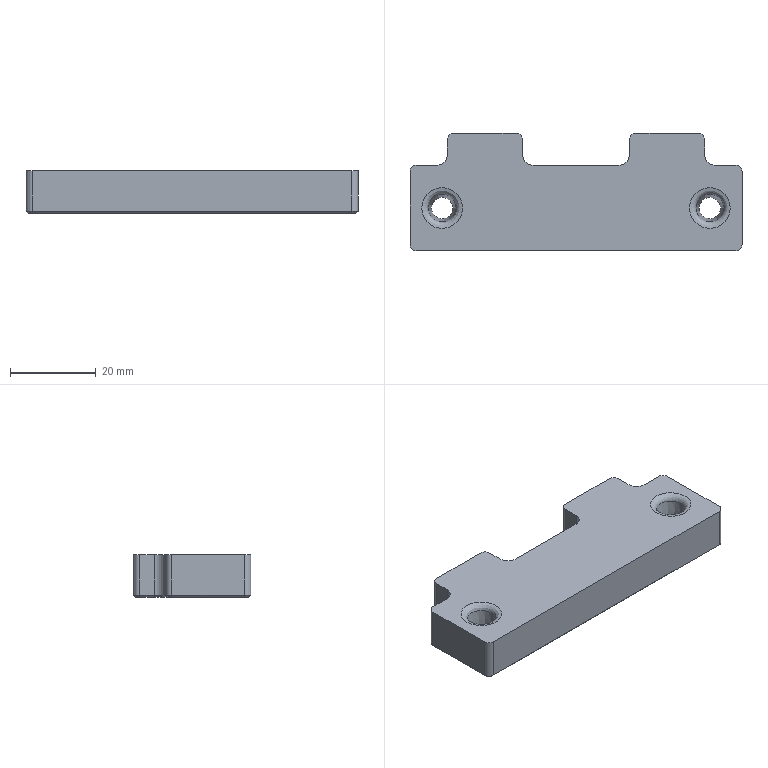Part | NX | features BLEND 3, DATUM_CSYS 3, EXTRUDE 2, SKETCH 2, CHAMFER 1, DRAFT 1, SCALE 1 | 1 solid | 54 faces | box 77.5 x 27.5 x 10 mm | volume 17549 mm3 | plane 26 | cone 14 | cylinder 12 | torus 2 | commonest cylinder face diameters 3 x8 5 x4
STEP:
#1=CARTESIAN_POINT('',(-38.75,8.5,10.));
#2=VERTEX_POINT('',#1);
#3=CARTESIAN_POINT('',(-38.75,8.5,0.5));
#4=VERTEX_POINT('',#3);
#5=CARTESIAN_POINT('',(-38.75,8.5,10.));
#6=DIRECTION('',(0.,0.,-1.));
#7=VECTOR('',#6,1000.);
#8=LINE('',#5,#7);
#9=EDGE_CURVE('',#2,#4,#8,.T.);
#10=ORIENTED_EDGE('',*,*,#9,.T.);
#11=CARTESIAN_POINT('',(-38.75,-8.5,0.5));
#12=VERTEX_POINT('',#11);
#13=CARTESIAN_POINT('',(-38.75,10.,0.5));
#14=DIRECTION('',(0.,-1.,0.));
#15=VECTOR('',#14,1000.);
#16=LINE('',#13,#15);
#17=EDGE_CURVE('',#4,#12,#16,.T.);
#18=ORIENTED_EDGE('',*,*,#17,.T.);
#19=CARTESIAN_POINT('',(-38.75,-8.5,10.));
#20=VERTEX_POINT('',#19);
#21=CARTESIAN_POINT('',(-38.75,-8.5,10.));
#22=DIRECTION('',(0.,0.,-1.));
#23=VECTOR('',#22,1000.);
#24=LINE('',#21,#23);
#25=EDGE_CURVE('',#12,#20,#24,.F.);
#26=ORIENTED_EDGE('',*,*,#25,.T.);
#27=CARTESIAN_POINT('',(-38.75,10.,10.));
#28=DIRECTION('',(0.,-1.,0.));
#29=VECTOR('',#28,1000.);
#30=LINE('',#27,#29);
#31=EDGE_CURVE('',#2,#20,#30,.T.);
#32=ORIENTED_EDGE('',*,*,#31,.F.);
#33=EDGE_LOOP('',(#10,#18,#26,#32));
#34=FACE_BOUND('',#33,.T.);
#35=CARTESIAN_POINT('',(-38.75,10.,10.));
#36=DIRECTION('',(1.,0.,0.));
#37=DIRECTION('',(0.,0.,-1.));
#38=AXIS2_PLACEMENT_3D('',#35,#36,#37);
#39=PLANE('',#38);
#40=ADVANCED_FACE('',(#34),#39,.F.);
#41=CARTESIAN_POINT('',(-37.25,-10.,10.));
#42=VERTEX_POINT('',#41);
#43=CARTESIAN_POINT('',(-37.25,-10.,0.5));
#44=VERTEX_POINT('',#43);
#45=CARTESIAN_POINT('',(-37.25,-10.,10.));
#46=DIRECTION('',(0.,0.,-1.));
#47=VECTOR('',#46,1000.);
#48=LINE('',#45,#47);
#49=EDGE_CURVE('',#42,#44,#48,.T.);
#50=ORIENTED_EDGE('',*,*,#49,.T.);
#51=CARTESIAN_POINT('',(37.25,-10.,0.5));
#52=VERTEX_POINT('',#51);
#53=CARTESIAN_POINT('',(-38.75,-10.,0.5));
#54=DIRECTION('',(1.,0.,0.));
#55=VECTOR('',#54,1000.);
#56=LINE('',#53,#55);
#57=EDGE_CURVE('',#44,#52,#56,.T.);
#58=ORIENTED_EDGE('',*,*,#57,.T.);
#59=CARTESIAN_POINT('',(37.25,-10.,10.));
#60=VERTEX_POINT('',#59);
#61=CARTESIAN_POINT('',(37.25,-10.,10.));
#62=DIRECTION('',(0.,0.,-1.));
#63=VECTOR('',#62,1000.);
#64=LINE('',#61,#63);
#65=EDGE_CURVE('',#52,#60,#64,.F.);
#66=ORIENTED_EDGE('',*,*,#65,.T.);
#67=CARTESIAN_POINT('',(-38.75,-10.,10.));
#68=DIRECTION('',(1.,0.,0.));
#69=VECTOR('',#68,1000.);
#70=LINE('',#67,#69);
#71=EDGE_CURVE('',#42,#60,#70,.T.);
#72=ORIENTED_EDGE('',*,*,#71,.F.);
#73=EDGE_LOOP('',(#50,#58,#66,#72));
#74=FACE_BOUND('',#73,.T.);
#75=CARTESIAN_POINT('',(-38.75,-10.,10.));
#76=DIRECTION('',(0.,1.,0.));
#77=DIRECTION('',(0.,0.,1.));
#78=AXIS2_PLACEMENT_3D('',#75,#76,#77);
#79=PLANE('',#78);
#80=ADVANCED_FACE('',(#74),#79,.F.);
#81=CARTESIAN_POINT('',(38.75,-8.5,10.));
#82=VERTEX_POINT('',#81);
#83=CARTESIAN_POINT('',(38.75,-8.5,0.5));
#84=VERTEX_POINT('',#83);
#85=CARTESIAN_POINT('',(38.75,-8.5,10.));
#86=DIRECTION('',(0.,0.,-1.));
#87=VECTOR('',#86,1000.);
#88=LINE('',#85,#87);
#89=EDGE_CURVE('',#82,#84,#88,.T.);
#90=ORIENTED_EDGE('',*,*,#89,.T.);
#91=CARTESIAN_POINT('',(38.75,8.5,0.5));
#92=VERTEX_POINT('',#91);
#93=CARTESIAN_POINT('',(38.75,-10.,0.5));
#94=DIRECTION('',(0.,1.,0.));
#95=VECTOR('',#94,1000.);
#96=LINE('',#93,#95);
#97=EDGE_CURVE('',#84,#92,#96,.T.);
#98=ORIENTED_EDGE('',*,*,#97,.T.);
#99=CARTESIAN_POINT('',(38.75,8.5,10.));
#100=VERTEX_POINT('',#99);
#101=CARTESIAN_POINT('',(38.75,8.5,10.));
#102=DIRECTION('',(0.,0.,-1.));
#103=VECTOR('',#102,1000.);
#104=LINE('',#101,#103);
#105=EDGE_CURVE('',#92,#100,#104,.F.);
#106=ORIENTED_EDGE('',*,*,#105,.T.);
#107=CARTESIAN_POINT('',(38.75,-10.,10.));
#108=DIRECTION('',(0.,1.,0.));
#109=VECTOR('',#108,1000.);
#110=LINE('',#107,#109);
#111=EDGE_CURVE('',#82,#100,#110,.T.);
#112=ORIENTED_EDGE('',*,*,#111,.F.);
#113=EDGE_LOOP('',(#90,#98,#106,#112));
#114=FACE_BOUND('',#113,.T.);
#115=CARTESIAN_POINT('',(38.75,-10.,10.));
#116=DIRECTION('',(-1.,0.,0.));
#117=DIRECTION('',(0.,0.,1.));
#118=AXIS2_PLACEMENT_3D('',#115,#116,#117);
#119=PLANE('',#118);
#120=ADVANCED_FACE('',(#114),#119,.F.);
#121=CARTESIAN_POINT('',(37.25,10.,10.));
#122=VERTEX_POINT('',#121);
#123=CARTESIAN_POINT('',(37.25,10.,0.5));
#124=VERTEX_POINT('',#123);
#125=CARTESIAN_POINT('',(37.25,10.,10.));
#126=DIRECTION('',(0.,0.,-1.));
#127=VECTOR('',#126,1000.);
#128=LINE('',#125,#127);
#129=EDGE_CURVE('',#122,#124,#128,.T.);
#130=ORIENTED_EDGE('',*,*,#129,.T.);
#131=CARTESIAN_POINT('',(32.5,10.,0.5));
#132=VERTEX_POINT('',#131);
#133=CARTESIAN_POINT('',(38.75,10.,0.5));
#134=DIRECTION('',(-1.,0.,0.));
#135=VECTOR('',#134,1000.);
#136=LINE('',#133,#135);
#137=EDGE_CURVE('',#124,#132,#136,.T.);
#138=ORIENTED_EDGE('',*,*,#137,.T.);
#139=CARTESIAN_POINT('',(32.5,10.,10.));
#140=VERTEX_POINT('',#139);
#141=CARTESIAN_POINT('',(32.5,10.,10.));
#142=DIRECTION('',(0.,0.,-1.));
#143=VECTOR('',#142,1000.);
#144=LINE('',#141,#143);
#145=EDGE_CURVE('',#132,#140,#144,.F.);
#146=ORIENTED_EDGE('',*,*,#145,.T.);
#147=CARTESIAN_POINT('',(38.75,10.,10.));
#148=DIRECTION('',(-1.,0.,0.));
#149=VECTOR('',#148,1000.);
#150=LINE('',#147,#149);
#151=EDGE_CURVE('',#122,#140,#150,.T.);
#152=ORIENTED_EDGE('',*,*,#151,.F.);
#153=EDGE_LOOP('',(#130,#138,#146,#152));
#154=FACE_BOUND('',#153,.T.);
#155=CARTESIAN_POINT('',(38.75,10.,10.));
#156=DIRECTION('',(0.,-1.,0.));
#157=DIRECTION('',(1.,0.,0.));
#158=AXIS2_PLACEMENT_3D('',#155,#156,#157);
#159=PLANE('',#158);
#160=ADVANCED_FACE('',(#154),#159,.F.);
#161=CARTESIAN_POINT('',(30.,12.5,10.));
#162=VERTEX_POINT('',#161);
#163=CARTESIAN_POINT('',(30.,12.5,0.5));
#164=VERTEX_POINT('',#163);
#165=CARTESIAN_POINT('',(30.,12.5,0.));
#166=DIRECTION('',(0.,0.,-1.));
#167=VECTOR('',#166,1000.);
#168=LINE('',#165,#167);
#169=EDGE_CURVE('',#162,#164,#168,.T.);
#170=ORIENTED_EDGE('',*,*,#169,.T.);
#171=CARTESIAN_POINT('',(30.,16.,0.5));
#172=VERTEX_POINT('',#171);
#173=CARTESIAN_POINT('',(30.,10.,0.5));
#174=DIRECTION('',(0.,1.,0.));
#175=VECTOR('',#174,1000.);
#176=LINE('',#173,#175);
#177=EDGE_CURVE('',#164,#172,#176,.T.);
#178=ORIENTED_EDGE('',*,*,#177,.T.);
#179=CARTESIAN_POINT('',(30.,16.,10.));
#180=VERTEX_POINT('',#179);
#181=CARTESIAN_POINT('',(30.,16.,10.));
#182=DIRECTION('',(0.,0.,-1.));
#183=VECTOR('',#182,1000.);
#184=LINE('',#181,#183);
#185=EDGE_CURVE('',#172,#180,#184,.F.);
#186=ORIENTED_EDGE('',*,*,#185,.T.);
#187=CARTESIAN_POINT('',(30.,10.,10.));
#188=DIRECTION('',(0.,1.,0.));
#189=VECTOR('',#188,1000.);
#190=LINE('',#187,#189);
#191=EDGE_CURVE('',#162,#180,#190,.T.);
#192=ORIENTED_EDGE('',*,*,#191,.F.);
#193=EDGE_LOOP('',(#170,#178,#186,#192));
#194=FACE_BOUND('',#193,.T.);
#195=CARTESIAN_POINT('',(30.,10.,10.));
#196=DIRECTION('',(-1.,0.,0.));
#197=DIRECTION('',(0.,0.,1.));
#198=AXIS2_PLACEMENT_3D('',#195,#196,#197);
#199=PLANE('',#198);
#200=ADVANCED_FACE('',(#194),#199,.F.);
#201=CARTESIAN_POINT('',(28.5,17.5,10.));
#202=VERTEX_POINT('',#201);
#203=CARTESIAN_POINT('',(28.5,17.5,0.5));
#204=VERTEX_POINT('',#203);
#205=CARTESIAN_POINT('',(28.5,17.5,10.));
#206=DIRECTION('',(0.,0.,-1.));
#207=VECTOR('',#206,1000.);
#208=LINE('',#205,#207);
#209=EDGE_CURVE('',#202,#204,#208,.T.);
#210=ORIENTED_EDGE('',*,*,#209,.T.);
#211=CARTESIAN_POINT('',(14.,17.5,0.5));
#212=VERTEX_POINT('',#211);
#213=CARTESIAN_POINT('',(30.,17.5,0.5));
#214=DIRECTION('',(-1.,0.,0.));
#215=VECTOR('',#214,1000.);
#216=LINE('',#213,#215);
#217=EDGE_CURVE('',#204,#212,#216,.T.);
#218=ORIENTED_EDGE('',*,*,#217,.T.);
#219=CARTESIAN_POINT('',(14.,17.5,10.));
#220=VERTEX_POINT('',#219);
#221=CARTESIAN_POINT('',(14.,17.5,10.));
#222=DIRECTION('',(0.,0.,-1.));
#223=VECTOR('',#222,1000.);
#224=LINE('',#221,#223);
#225=EDGE_CURVE('',#212,#220,#224,.F.);
#226=ORIENTED_EDGE('',*,*,#225,.T.);
#227=CARTESIAN_POINT('',(30.,17.5,10.));
#228=DIRECTION('',(-1.,0.,0.));
#229=VECTOR('',#228,1000.);
#230=LINE('',#227,#229);
#231=EDGE_CURVE('',#202,#220,#230,.T.);
#232=ORIENTED_EDGE('',*,*,#231,.F.);
#233=EDGE_LOOP('',(#210,#218,#226,#232));
#234=FACE_BOUND('',#233,.T.);
#235=CARTESIAN_POINT('',(30.,17.5,10.));
#236=DIRECTION('',(0.,-1.,0.));
#237=DIRECTION('',(1.,0.,0.));
#238=AXIS2_PLACEMENT_3D('',#235,#236,#237);
#239=PLANE('',#238);
#240=ADVANCED_FACE('',(#234),#239,.F.);
#241=CARTESIAN_POINT('',(12.5,16.,10.));
#242=VERTEX_POINT('',#241);
#243=CARTESIAN_POINT('',(12.5,16.,0.5));
#244=VERTEX_POINT('',#243);
#245=CARTESIAN_POINT('',(12.5,16.,10.));
#246=DIRECTION('',(0.,0.,-1.));
#247=VECTOR('',#246,1000.);
#248=LINE('',#245,#247);
#249=EDGE_CURVE('',#242,#244,#248,.T.);
#250=ORIENTED_EDGE('',*,*,#249,.T.);
#251=CARTESIAN_POINT('',(12.5,12.5,0.5));
#252=VERTEX_POINT('',#251);
#253=CARTESIAN_POINT('',(12.5,17.5,0.5));
#254=DIRECTION('',(0.,-1.,0.));
#255=VECTOR('',#254,1000.);
#256=LINE('',#253,#255);
#257=EDGE_CURVE('',#244,#252,#256,.T.);
#258=ORIENTED_EDGE('',*,*,#257,.T.);
#259=CARTESIAN_POINT('',(12.5,12.5,10.));
#260=VERTEX_POINT('',#259);
#261=CARTESIAN_POINT('',(12.5,12.5,10.));
#262=DIRECTION('',(0.,0.,-1.));
#263=VECTOR('',#262,1000.);
#264=LINE('',#261,#263);
#265=EDGE_CURVE('',#252,#260,#264,.F.);
#266=ORIENTED_EDGE('',*,*,#265,.T.);
#267=CARTESIAN_POINT('',(12.5,17.5,10.));
#268=DIRECTION('',(0.,-1.,0.));
#269=VECTOR('',#268,1000.);
#270=LINE('',#267,#269);
#271=EDGE_CURVE('',#242,#260,#270,.T.);
#272=ORIENTED_EDGE('',*,*,#271,.F.);
#273=EDGE_LOOP('',(#250,#258,#266,#272));
#274=FACE_BOUND('',#273,.T.);
#275=CARTESIAN_POINT('',(12.5,17.5,10.));
#276=DIRECTION('',(1.,0.,0.));
#277=DIRECTION('',(0.,0.,-1.));
#278=AXIS2_PLACEMENT_3D('',#275,#276,#277);
#279=PLANE('',#278);
#280=ADVANCED_FACE('',(#274),#279,.F.);
#281=CARTESIAN_POINT('',(10.,10.,10.));
#282=VERTEX_POINT('',#281);
#283=CARTESIAN_POINT('',(10.,10.,0.5));
#284=VERTEX_POINT('',#283);
#285=CARTESIAN_POINT('',(10.,10.,0.));
#286=DIRECTION('',(0.,0.,-1.));
#287=VECTOR('',#286,1000.);
#288=LINE('',#285,#287);
#289=EDGE_CURVE('',#282,#284,#288,.T.);
#290=ORIENTED_EDGE('',*,*,#289,.T.);
#291=CARTESIAN_POINT('',(-10.,10.,0.5));
#292=VERTEX_POINT('',#291);
#293=CARTESIAN_POINT('',(12.5,10.,0.5));
#294=DIRECTION('',(-1.,0.,0.));
#295=VECTOR('',#294,1000.);
#296=LINE('',#293,#295);
#297=EDGE_CURVE('',#284,#292,#296,.T.);
#298=ORIENTED_EDGE('',*,*,#297,.T.);
#299=CARTESIAN_POINT('',(-10.,10.,10.));
#300=VERTEX_POINT('',#299);
#301=CARTESIAN_POINT('',(-10.,10.,10.));
#302=DIRECTION('',(0.,0.,-1.));
#303=VECTOR('',#302,1000.);
#304=LINE('',#301,#303);
#305=EDGE_CURVE('',#292,#300,#304,.F.);
#306=ORIENTED_EDGE('',*,*,#305,.T.);
#307=CARTESIAN_POINT('',(12.5,10.,10.));
#308=DIRECTION('',(-1.,0.,0.));
#309=VECTOR('',#308,1000.);
#310=LINE('',#307,#309);
#311=EDGE_CURVE('',#282,#300,#310,.T.);
#312=ORIENTED_EDGE('',*,*,#311,.F.);
#313=EDGE_LOOP('',(#290,#298,#306,#312));
#314=FACE_BOUND('',#313,.T.);
#315=CARTESIAN_POINT('',(12.5,10.,10.));
#316=DIRECTION('',(0.,-1.,0.));
#317=DIRECTION('',(0.,0.,-1.));
#318=AXIS2_PLACEMENT_3D('',#315,#316,#317);
#319=PLANE('',#318);
#320=ADVANCED_FACE('',(#314),#319,.F.);
#321=CARTESIAN_POINT('',(-12.5,12.5,10.));
#322=VERTEX_POINT('',#321);
#323=CARTESIAN_POINT('',(-12.5,12.5,0.5));
#324=VERTEX_POINT('',#323);
#325=CARTESIAN_POINT('',(-12.5,12.5,0.));
#326=DIRECTION('',(0.,0.,-1.));
#327=VECTOR('',#326,1000.);
#328=LINE('',#325,#327);
#329=EDGE_CURVE('',#322,#324,#328,.T.);
#330=ORIENTED_EDGE('',*,*,#329,.T.);
#331=CARTESIAN_POINT('',(-12.5,16.,0.5));
#332=VERTEX_POINT('',#331);
#333=CARTESIAN_POINT('',(-12.5,10.,0.5));
#334=DIRECTION('',(0.,1.,0.));
#335=VECTOR('',#334,1000.);
#336=LINE('',#333,#335);
#337=EDGE_CURVE('',#324,#332,#336,.T.);
#338=ORIENTED_EDGE('',*,*,#337,.T.);
#339=CARTESIAN_POINT('',(-12.5,16.,10.));
#340=VERTEX_POINT('',#339);
#341=CARTESIAN_POINT('',(-12.5,16.,10.));
#342=DIRECTION('',(0.,0.,-1.));
#343=VECTOR('',#342,1000.);
#344=LINE('',#341,#343);
#345=EDGE_CURVE('',#332,#340,#344,.F.);
#346=ORIENTED_EDGE('',*,*,#345,.T.);
#347=CARTESIAN_POINT('',(-12.5,10.,10.));
#348=DIRECTION('',(0.,1.,0.));
#349=VECTOR('',#348,1000.);
#350=LINE('',#347,#349);
#351=EDGE_CURVE('',#322,#340,#350,.T.);
#352=ORIENTED_EDGE('',*,*,#351,.F.);
#353=EDGE_LOOP('',(#330,#338,#346,#352));
#354=FACE_BOUND('',#353,.T.);
#355=CARTESIAN_POINT('',(-12.5,10.,10.));
#356=DIRECTION('',(-1.,0.,0.));
#357=DIRECTION('',(0.,0.,1.));
#358=AXIS2_PLACEMENT_3D('',#355,#356,#357);
#359=PLANE('',#358);
#360=ADVANCED_FACE('',(#354),#359,.F.);
#361=CARTESIAN_POINT('',(-14.,17.5,10.));
#362=VERTEX_POINT('',#361);
#363=CARTESIAN_POINT('',(-14.,17.5,0.5));
#364=VERTEX_POINT('',#363);
#365=CARTESIAN_POINT('',(-14.,17.5,10.));
#366=DIRECTION('',(0.,0.,-1.));
#367=VECTOR('',#366,1000.);
#368=LINE('',#365,#367);
#369=EDGE_CURVE('',#362,#364,#368,.T.);
#370=ORIENTED_EDGE('',*,*,#369,.T.);
#371=CARTESIAN_POINT('',(-28.5,17.5,0.5));
#372=VERTEX_POINT('',#371);
#373=CARTESIAN_POINT('',(-12.5,17.5,0.5));
#374=DIRECTION('',(-1.,0.,0.));
#375=VECTOR('',#374,1000.);
#376=LINE('',#373,#375);
#377=EDGE_CURVE('',#364,#372,#376,.T.);
#378=ORIENTED_EDGE('',*,*,#377,.T.);
#379=CARTESIAN_POINT('',(-28.5,17.5,10.));
#380=VERTEX_POINT('',#379);
#381=CARTESIAN_POINT('',(-28.5,17.5,10.));
#382=DIRECTION('',(0.,0.,-1.));
#383=VECTOR('',#382,1000.);
#384=LINE('',#381,#383);
#385=EDGE_CURVE('',#372,#380,#384,.F.);
#386=ORIENTED_EDGE('',*,*,#385,.T.);
#387=CARTESIAN_POINT('',(-12.5,17.5,10.));
#388=DIRECTION('',(-1.,0.,0.));
#389=VECTOR('',#388,1000.);
#390=LINE('',#387,#389);
#391=EDGE_CURVE('',#362,#380,#390,.T.);
#392=ORIENTED_EDGE('',*,*,#391,.F.);
#393=EDGE_LOOP('',(#370,#378,#386,#392));
#394=FACE_BOUND('',#393,.T.);
#395=CARTESIAN_POINT('',(-12.5,17.5,10.));
#396=DIRECTION('',(0.,-1.,0.));
#397=DIRECTION('',(1.,0.,0.));
#398=AXIS2_PLACEMENT_3D('',#395,#396,#397);
#399=PLANE('',#398);
#400=ADVANCED_FACE('',(#394),#399,.F.);
#401=CARTESIAN_POINT('',(-30.,16.,10.));
#402=VERTEX_POINT('',#401);
#403=CARTESIAN_POINT('',(-30.,16.,0.5));
#404=VERTEX_POINT('',#403);
#405=CARTESIAN_POINT('',(-30.,16.,10.));
#406=DIRECTION('',(0.,0.,-1.));
#407=VECTOR('',#406,1000.);
#408=LINE('',#405,#407);
#409=EDGE_CURVE('',#402,#404,#408,.T.);
#410=ORIENTED_EDGE('',*,*,#409,.T.);
#411=CARTESIAN_POINT('',(-30.,12.5,0.5));
#412=VERTEX_POINT('',#411);
#413=CARTESIAN_POINT('',(-30.,17.5,0.5));
#414=DIRECTION('',(0.,-1.,0.));
#415=VECTOR('',#414,1000.);
#416=LINE('',#413,#415);
#417=EDGE_CURVE('',#404,#412,#416,.T.);
#418=ORIENTED_EDGE('',*,*,#417,.T.);
#419=CARTESIAN_POINT('',(-30.,12.5,10.));
#420=VERTEX_POINT('',#419);
#421=CARTESIAN_POINT('',(-30.,12.5,10.));
#422=DIRECTION('',(0.,0.,-1.));
#423=VECTOR('',#422,1000.);
#424=LINE('',#421,#423);
#425=EDGE_CURVE('',#412,#420,#424,.F.);
#426=ORIENTED_EDGE('',*,*,#425,.T.);
#427=CARTESIAN_POINT('',(-30.,17.5,10.));
#428=DIRECTION('',(0.,-1.,0.));
#429=VECTOR('',#428,1000.);
#430=LINE('',#427,#429);
#431=EDGE_CURVE('',#402,#420,#430,.T.);
#432=ORIENTED_EDGE('',*,*,#431,.F.);
#433=EDGE_LOOP('',(#410,#418,#426,#432));
#434=FACE_BOUND('',#433,.T.);
#435=CARTESIAN_POINT('',(-30.,17.5,10.));
#436=DIRECTION('',(1.,0.,0.));
#437=DIRECTION('',(0.,0.,-1.));
#438=AXIS2_PLACEMENT_3D('',#435,#436,#437);
#439=PLANE('',#438);
#440=ADVANCED_FACE('',(#434),#439,.F.);
#441=CARTESIAN_POINT('',(-32.5,10.,10.));
#442=VERTEX_POINT('',#441);
#443=CARTESIAN_POINT('',(-32.5,10.,0.5));
#444=VERTEX_POINT('',#443);
#445=CARTESIAN_POINT('',(-32.5,10.,0.));
#446=DIRECTION('',(0.,0.,-1.));
#447=VECTOR('',#446,1000.);
#448=LINE('',#445,#447);
#449=EDGE_CURVE('',#442,#444,#448,.T.);
#450=ORIENTED_EDGE('',*,*,#449,.T.);
#451=CARTESIAN_POINT('',(-37.25,10.,0.5));
#452=VERTEX_POINT('',#451);
#453=CARTESIAN_POINT('',(-30.,10.,0.5));
#454=DIRECTION('',(-1.,0.,0.));
#455=VECTOR('',#454,1000.);
#456=LINE('',#453,#455);
#457=EDGE_CURVE('',#444,#452,#456,.T.);
#458=ORIENTED_EDGE('',*,*,#457,.T.);
#459=CARTESIAN_POINT('',(-37.25,10.,10.));
#460=VERTEX_POINT('',#459);
#461=CARTESIAN_POINT('',(-37.25,10.,10.));
#462=DIRECTION('',(0.,0.,-1.));
#463=VECTOR('',#462,1000.);
#464=LINE('',#461,#463);
#465=EDGE_CURVE('',#452,#460,#464,.F.);
#466=ORIENTED_EDGE('',*,*,#465,.T.);
#467=CARTESIAN_POINT('',(-30.,10.,10.));
#468=DIRECTION('',(-1.,0.,0.));
#469=VECTOR('',#468,1000.);
#470=LINE('',#467,#469);
#471=EDGE_CURVE('',#442,#460,#470,.T.);
#472=ORIENTED_EDGE('',*,*,#471,.F.);
#473=EDGE_LOOP('',(#450,#458,#466,#472));
#474=FACE_BOUND('',#473,.T.);
#475=CARTESIAN_POINT('',(-30.,10.,10.));
#476=DIRECTION('',(0.,-1.,0.));
#477=DIRECTION('',(1.,0.,0.));
#478=AXIS2_PLACEMENT_3D('',#475,#476,#477);
#479=PLANE('',#478);
#480=ADVANCED_FACE('',(#474),#479,.F.);
#481=CARTESIAN_POINT('',(35.999,0.,10.));
#482=VERTEX_POINT('',#481);
#483=CARTESIAN_POINT('',(31.25,0.,10.));
#484=DIRECTION('',(0.,0.,1.));
#485=DIRECTION('',(1.,0.,0.));
#486=AXIS2_PLACEMENT_3D('',#483,#484,#485);
#487=CIRCLE('',#486,4.749);
#488=EDGE_CURVE('',#482,#482,#487,.F.);
#489=ORIENTED_EDGE('',*,*,#488,.T.);
#490=EDGE_LOOP('',(#489));
#491=FACE_BOUND('',#490,.T.);
#492=CARTESIAN_POINT('',(-26.501,0.,10.));
#493=VERTEX_POINT('',#492);
#494=CARTESIAN_POINT('',(-31.25,0.,10.));
#495=DIRECTION('',(0.,0.,1.));
#496=DIRECTION('',(1.,0.,0.));
#497=AXIS2_PLACEMENT_3D('',#494,#495,#496);
#498=CIRCLE('',#497,4.749);
#499=EDGE_CURVE('',#493,#493,#498,.F.);
#500=ORIENTED_EDGE('',*,*,#499,.T.);
#501=EDGE_LOOP('',(#500));
#502=FACE_BOUND('',#501,.T.);
#503=ORIENTED_EDGE('',*,*,#31,.T.);
#504=CARTESIAN_POINT('',(-37.25,-8.5,10.));
#505=DIRECTION('',(0.,0.,1.));
#506=DIRECTION('',(1.,0.,0.));
#507=AXIS2_PLACEMENT_3D('',#504,#505,#506);
#508=CIRCLE('',#507,1.5);
#509=EDGE_CURVE('',#20,#42,#508,.T.);
#510=ORIENTED_EDGE('',*,*,#509,.T.);
#511=ORIENTED_EDGE('',*,*,#71,.T.);
#512=CARTESIAN_POINT('',(37.25,-8.5,10.));
#513=DIRECTION('',(0.,0.,1.));
#514=DIRECTION('',(1.,0.,0.));
#515=AXIS2_PLACEMENT_3D('',#512,#513,#514);
#516=CIRCLE('',#515,1.5);
#517=EDGE_CURVE('',#60,#82,#516,.T.);
#518=ORIENTED_EDGE('',*,*,#517,.T.);
#519=ORIENTED_EDGE('',*,*,#111,.T.);
#520=CARTESIAN_POINT('',(37.25,8.5,10.));
#521=DIRECTION('',(0.,0.,1.));
#522=DIRECTION('',(1.,0.,0.));
#523=AXIS2_PLACEMENT_3D('',#520,#521,#522);
#524=CIRCLE('',#523,1.5);
#525=EDGE_CURVE('',#100,#122,#524,.T.);
#526=ORIENTED_EDGE('',*,*,#525,.T.);
#527=ORIENTED_EDGE('',*,*,#151,.T.);
#528=CARTESIAN_POINT('',(32.5,12.5,10.));
#529=DIRECTION('',(0.,0.,1.));
#530=DIRECTION('',(1.,0.,0.));
#531=AXIS2_PLACEMENT_3D('',#528,#529,#530);
#532=CIRCLE('',#531,2.5);
#533=EDGE_CURVE('',#140,#162,#532,.F.);
#534=ORIENTED_EDGE('',*,*,#533,.T.);
#535=ORIENTED_EDGE('',*,*,#191,.T.);
#536=CARTESIAN_POINT('',(28.5,16.,10.));
#537=DIRECTION('',(0.,0.,1.));
#538=DIRECTION('',(1.,0.,0.));
#539=AXIS2_PLACEMENT_3D('',#536,#537,#538);
#540=CIRCLE('',#539,1.5);
#541=EDGE_CURVE('',#180,#202,#540,.T.);
#542=ORIENTED_EDGE('',*,*,#541,.T.);
#543=ORIENTED_EDGE('',*,*,#231,.T.);
#544=CARTESIAN_POINT('',(14.,16.,10.));
#545=DIRECTION('',(0.,0.,1.));
#546=DIRECTION('',(1.,0.,0.));
#547=AXIS2_PLACEMENT_3D('',#544,#545,#546);
#548=CIRCLE('',#547,1.5);
#549=EDGE_CURVE('',#220,#242,#548,.T.);
#550=ORIENTED_EDGE('',*,*,#549,.T.);
#551=ORIENTED_EDGE('',*,*,#271,.T.);
#552=CARTESIAN_POINT('',(10.,12.5,10.));
#553=DIRECTION('',(0.,0.,1.));
#554=DIRECTION('',(1.,0.,0.));
#555=AXIS2_PLACEMENT_3D('',#552,#553,#554);
#556=CIRCLE('',#555,2.5);
#557=EDGE_CURVE('',#260,#282,#556,.F.);
#558=ORIENTED_EDGE('',*,*,#557,.T.);
#559=ORIENTED_EDGE('',*,*,#311,.T.);
#560=CARTESIAN_POINT('',(-10.,12.5,10.));
#561=DIRECTION('',(0.,0.,1.));
#562=DIRECTION('',(1.,0.,0.));
#563=AXIS2_PLACEMENT_3D('',#560,#561,#562);
#564=CIRCLE('',#563,2.5);
#565=EDGE_CURVE('',#300,#322,#564,.F.);
#566=ORIENTED_EDGE('',*,*,#565,.T.);
#567=ORIENTED_EDGE('',*,*,#351,.T.);
#568=CARTESIAN_POINT('',(-14.,16.,10.));
#569=DIRECTION('',(0.,0.,1.));
#570=DIRECTION('',(1.,0.,0.));
#571=AXIS2_PLACEMENT_3D('',#568,#569,#570);
#572=CIRCLE('',#571,1.5);
#573=EDGE_CURVE('',#340,#362,#572,.T.);
#574=ORIENTED_EDGE('',*,*,#573,.T.);
#575=ORIENTED_EDGE('',*,*,#391,.T.);
#576=CARTESIAN_POINT('',(-28.5,16.,10.));
#577=DIRECTION('',(0.,0.,1.));
#578=DIRECTION('',(1.,0.,0.));
#579=AXIS2_PLACEMENT_3D('',#576,#577,#578);
#580=CIRCLE('',#579,1.5);
#581=EDGE_CURVE('',#380,#402,#580,.T.);
#582=ORIENTED_EDGE('',*,*,#581,.T.);
#583=ORIENTED_EDGE('',*,*,#431,.T.);
#584=CARTESIAN_POINT('',(-32.5,12.5,10.));
#585=DIRECTION('',(0.,0.,1.));
#586=DIRECTION('',(1.,0.,0.));
#587=AXIS2_PLACEMENT_3D('',#584,#585,#586);
#588=CIRCLE('',#587,2.5);
#589=EDGE_CURVE('',#420,#442,#588,.F.);
#590=ORIENTED_EDGE('',*,*,#589,.T.);
#591=ORIENTED_EDGE('',*,*,#471,.T.);
#592=CARTESIAN_POINT('',(-37.25,8.5,10.));
#593=DIRECTION('',(0.,0.,1.));
#594=DIRECTION('',(1.,0.,0.));
#595=AXIS2_PLACEMENT_3D('',#592,#593,#594);
#596=CIRCLE('',#595,1.5);
#597=EDGE_CURVE('',#460,#2,#596,.T.);
#598=ORIENTED_EDGE('',*,*,#597,.T.);
#599=EDGE_LOOP('',(#503,#510,#511,#518,#519,#526,#527,#534,#535,#542,#543,#550,#551,#558,#559,#566,#567,#574,#575,#582,#583,#590,#591,#598));
#600=FACE_BOUND('',#599,.T.);
#601=CARTESIAN_POINT('',(0.,0.,10.));
#602=DIRECTION('',(0.,0.,1.));
#603=DIRECTION('',(1.,0.,0.));
#604=AXIS2_PLACEMENT_3D('',#601,#602,#603);
#605=PLANE('',#604);
#606=ADVANCED_FACE('',(#491,#502,#600),#605,.T.);
#607=CARTESIAN_POINT('',(37.25,-9.5,0.));
#608=VERTEX_POINT('',#607);
#609=CARTESIAN_POINT('',(-37.25,-9.5,0.));
#610=VERTEX_POINT('',#609);
#611=CARTESIAN_POINT('',(0.,-9.5,0.));
#612=DIRECTION('',(-1.,0.,0.));
#613=VECTOR('',#612,1000.);
#614=LINE('',#611,#613);
#615=EDGE_CURVE('',#608,#610,#614,.T.);
#616=ORIENTED_EDGE('',*,*,#615,.T.);
#617=CARTESIAN_POINT('',(-38.25,-8.5,0.));
#618=VERTEX_POINT('',#617);
#619=CARTESIAN_POINT('',(-37.25,-8.5,0.));
#620=DIRECTION('',(0.,0.,1.));
#621=DIRECTION('',(1.,0.,0.));
#622=AXIS2_PLACEMENT_3D('',#619,#620,#621);
#623=CIRCLE('',#622,1.);
#624=EDGE_CURVE('',#610,#618,#623,.F.);
#625=ORIENTED_EDGE('',*,*,#624,.T.);
#626=CARTESIAN_POINT('',(-38.25,8.5,0.));
#627=VERTEX_POINT('',#626);
#628=CARTESIAN_POINT('',(-38.25,0.,0.));
#629=DIRECTION('',(0.,1.,0.));
#630=VECTOR('',#629,1000.);
#631=LINE('',#628,#630);
#632=EDGE_CURVE('',#618,#627,#631,.T.);
#633=ORIENTED_EDGE('',*,*,#632,.T.);
#634=CARTESIAN_POINT('',(-37.25,9.5,0.));
#635=VERTEX_POINT('',#634);
#636=CARTESIAN_POINT('',(-37.25,8.5,0.));
#637=DIRECTION('',(0.,0.,1.));
#638=DIRECTION('',(1.,0.,0.));
#639=AXIS2_PLACEMENT_3D('',#636,#637,#638);
#640=CIRCLE('',#639,1.);
#641=EDGE_CURVE('',#627,#635,#640,.F.);
#642=ORIENTED_EDGE('',*,*,#641,.T.);
#643=CARTESIAN_POINT('',(-32.5,9.5,0.));
#644=VERTEX_POINT('',#643);
#645=CARTESIAN_POINT('',(0.,9.5,0.));
#646=DIRECTION('',(1.,0.,0.));
#647=VECTOR('',#646,1000.);
#648=LINE('',#645,#647);
#649=EDGE_CURVE('',#635,#644,#648,.T.);
#650=ORIENTED_EDGE('',*,*,#649,.T.);
#651=CARTESIAN_POINT('',(-29.5,12.5,0.));
#652=VERTEX_POINT('',#651);
#653=CARTESIAN_POINT('',(-32.5,12.5,0.));
#654=DIRECTION('',(0.,0.,1.));
#655=DIRECTION('',(1.,0.,0.));
#656=AXIS2_PLACEMENT_3D('',#653,#654,#655);
#657=CIRCLE('',#656,3.);
#658=EDGE_CURVE('',#644,#652,#657,.T.);
#659=ORIENTED_EDGE('',*,*,#658,.T.);
#660=CARTESIAN_POINT('',(-29.5,16.,0.));
#661=VERTEX_POINT('',#660);
#662=CARTESIAN_POINT('',(-29.5,0.,0.));
#663=DIRECTION('',(0.,1.,0.));
#664=VECTOR('',#663,1000.);
#665=LINE('',#662,#664);
#666=EDGE_CURVE('',#652,#661,#665,.T.);
#667=ORIENTED_EDGE('',*,*,#666,.T.);
#668=CARTESIAN_POINT('',(-28.5,17.,0.));
#669=VERTEX_POINT('',#668);
#670=CARTESIAN_POINT('',(-28.5,16.,0.));
#671=DIRECTION('',(0.,0.,1.));
#672=DIRECTION('',(1.,0.,0.));
#673=AXIS2_PLACEMENT_3D('',#670,#671,#672);
#674=CIRCLE('',#673,1.);
#675=EDGE_CURVE('',#661,#669,#674,.F.);
#676=ORIENTED_EDGE('',*,*,#675,.T.);
#677=CARTESIAN_POINT('',(-14.,17.,0.));
#678=VERTEX_POINT('',#677);
#679=CARTESIAN_POINT('',(0.,17.,0.));
#680=DIRECTION('',(1.,0.,0.));
#681=VECTOR('',#680,1000.);
#682=LINE('',#679,#681);
#683=EDGE_CURVE('',#669,#678,#682,.T.);
#684=ORIENTED_EDGE('',*,*,#683,.T.);
#685=CARTESIAN_POINT('',(-13.,16.,0.));
#686=VERTEX_POINT('',#685);
#687=CARTESIAN_POINT('',(-14.,16.,0.));
#688=DIRECTION('',(0.,0.,1.));
#689=DIRECTION('',(1.,0.,0.));
#690=AXIS2_PLACEMENT_3D('',#687,#688,#689);
#691=CIRCLE('',#690,1.);
#692=EDGE_CURVE('',#678,#686,#691,.F.);
#693=ORIENTED_EDGE('',*,*,#692,.T.);
#694=CARTESIAN_POINT('',(-13.,12.5,0.));
#695=VERTEX_POINT('',#694);
#696=CARTESIAN_POINT('',(-13.,0.,0.));
#697=DIRECTION('',(0.,-1.,0.));
#698=VECTOR('',#697,1000.);
#699=LINE('',#696,#698);
#700=EDGE_CURVE('',#686,#695,#699,.T.);
#701=ORIENTED_EDGE('',*,*,#700,.T.);
#702=CARTESIAN_POINT('',(-10.,9.5,0.));
#703=VERTEX_POINT('',#702);
#704=CARTESIAN_POINT('',(-10.,12.5,0.));
#705=DIRECTION('',(0.,0.,1.));
#706=DIRECTION('',(1.,0.,0.));
#707=AXIS2_PLACEMENT_3D('',#704,#705,#706);
#708=CIRCLE('',#707,3.);
#709=EDGE_CURVE('',#695,#703,#708,.T.);
#710=ORIENTED_EDGE('',*,*,#709,.T.);
#711=CARTESIAN_POINT('',(10.,9.5,0.));
#712=VERTEX_POINT('',#711);
#713=CARTESIAN_POINT('',(0.,9.5,0.));
#714=DIRECTION('',(1.,0.,0.));
#715=VECTOR('',#714,1000.);
#716=LINE('',#713,#715);
#717=EDGE_CURVE('',#703,#712,#716,.T.);
#718=ORIENTED_EDGE('',*,*,#717,.T.);
#719=CARTESIAN_POINT('',(13.,12.5,0.));
#720=VERTEX_POINT('',#719);
#721=CARTESIAN_POINT('',(10.,12.5,0.));
#722=DIRECTION('',(0.,0.,1.));
#723=DIRECTION('',(1.,0.,0.));
#724=AXIS2_PLACEMENT_3D('',#721,#722,#723);
#725=CIRCLE('',#724,3.);
#726=EDGE_CURVE('',#712,#720,#725,.T.);
#727=ORIENTED_EDGE('',*,*,#726,.T.);
#728=CARTESIAN_POINT('',(13.,16.,0.));
#729=VERTEX_POINT('',#728);
#730=CARTESIAN_POINT('',(13.,0.,0.));
#731=DIRECTION('',(0.,1.,0.));
#732=VECTOR('',#731,1000.);
#733=LINE('',#730,#732);
#734=EDGE_CURVE('',#720,#729,#733,.T.);
#735=ORIENTED_EDGE('',*,*,#734,.T.);
#736=CARTESIAN_POINT('',(14.,17.,0.));
#737=VERTEX_POINT('',#736);
#738=CARTESIAN_POINT('',(14.,16.,0.));
#739=DIRECTION('',(0.,0.,1.));
#740=DIRECTION('',(1.,0.,0.));
#741=AXIS2_PLACEMENT_3D('',#738,#739,#740);
#742=CIRCLE('',#741,1.);
#743=EDGE_CURVE('',#729,#737,#742,.F.);
#744=ORIENTED_EDGE('',*,*,#743,.T.);
#745=CARTESIAN_POINT('',(28.5,17.,0.));
#746=VERTEX_POINT('',#745);
#747=CARTESIAN_POINT('',(0.,17.,0.));
#748=DIRECTION('',(1.,0.,0.));
#749=VECTOR('',#748,1000.);
#750=LINE('',#747,#749);
#751=EDGE_CURVE('',#737,#746,#750,.T.);
#752=ORIENTED_EDGE('',*,*,#751,.T.);
#753=CARTESIAN_POINT('',(29.5,16.,0.));
#754=VERTEX_POINT('',#753);
#755=CARTESIAN_POINT('',(28.5,16.,0.));
#756=DIRECTION('',(0.,0.,1.));
#757=DIRECTION('',(1.,0.,0.));
#758=AXIS2_PLACEMENT_3D('',#755,#756,#757);
#759=CIRCLE('',#758,1.);
#760=EDGE_CURVE('',#746,#754,#759,.F.);
#761=ORIENTED_EDGE('',*,*,#760,.T.);
#762=CARTESIAN_POINT('',(29.5,12.5,0.));
#763=VERTEX_POINT('',#762);
#764=CARTESIAN_POINT('',(29.5,0.,0.));
#765=DIRECTION('',(0.,-1.,0.));
#766=VECTOR('',#765,1000.);
#767=LINE('',#764,#766);
#768=EDGE_CURVE('',#754,#763,#767,.T.);
#769=ORIENTED_EDGE('',*,*,#768,.T.);
#770=CARTESIAN_POINT('',(32.5,9.5,0.));
#771=VERTEX_POINT('',#770);
#772=CARTESIAN_POINT('',(32.5,12.5,0.));
#773=DIRECTION('',(0.,0.,1.));
#774=DIRECTION('',(1.,0.,0.));
#775=AXIS2_PLACEMENT_3D('',#772,#773,#774);
#776=CIRCLE('',#775,3.);
#777=EDGE_CURVE('',#763,#771,#776,.T.);
#778=ORIENTED_EDGE('',*,*,#777,.T.);
#779=CARTESIAN_POINT('',(37.25,9.5,0.));
#780=VERTEX_POINT('',#779);
#781=CARTESIAN_POINT('',(0.,9.5,0.));
#782=DIRECTION('',(1.,0.,0.));
#783=VECTOR('',#782,1000.);
#784=LINE('',#781,#783);
#785=EDGE_CURVE('',#771,#780,#784,.T.);
#786=ORIENTED_EDGE('',*,*,#785,.T.);
#787=CARTESIAN_POINT('',(38.25,8.5,0.));
#788=VERTEX_POINT('',#787);
#789=CARTESIAN_POINT('',(37.25,8.5,0.));
#790=DIRECTION('',(0.,0.,1.));
#791=DIRECTION('',(1.,0.,0.));
#792=AXIS2_PLACEMENT_3D('',#789,#790,#791);
#793=CIRCLE('',#792,1.);
#794=EDGE_CURVE('',#780,#788,#793,.F.);
#795=ORIENTED_EDGE('',*,*,#794,.T.);
#796=CARTESIAN_POINT('',(38.25,-8.5,0.));
#797=VERTEX_POINT('',#796);
#798=CARTESIAN_POINT('',(38.25,0.,0.));
#799=DIRECTION('',(0.,-1.,0.));
#800=VECTOR('',#799,1000.);
#801=LINE('',#798,#800);
#802=EDGE_CURVE('',#788,#797,#801,.T.);
#803=ORIENTED_EDGE('',*,*,#802,.T.);
#804=CARTESIAN_POINT('',(37.25,-8.5,0.));
#805=DIRECTION('',(0.,0.,1.));
#806=DIRECTION('',(1.,0.,0.));
#807=AXIS2_PLACEMENT_3D('',#804,#805,#806);
#808=CIRCLE('',#807,1.);
#809=EDGE_CURVE('',#797,#608,#808,.F.);
#810=ORIENTED_EDGE('',*,*,#809,.T.);
#811=EDGE_LOOP('',(#616,#625,#633,#642,#650,#659,#667,#676,#684,#693,#701,#710,#718,#727,#735,#744,#752,#761,#769,#778,#786,#795,#803,#810));
#812=FACE_BOUND('',#811,.T.);
#813=CARTESIAN_POINT('',(-28.75,0.,0.));
#814=VERTEX_POINT('',#813);
#815=CARTESIAN_POINT('',(-31.25,0.,0.));
#816=DIRECTION('',(0.,0.,1.));
#817=DIRECTION('',(1.,0.,0.));
#818=AXIS2_PLACEMENT_3D('',#815,#816,#817);
#819=CIRCLE('',#818,2.5);
#820=EDGE_CURVE('',#814,#814,#819,.T.);
#821=ORIENTED_EDGE('',*,*,#820,.T.);
#822=EDGE_LOOP('',(#821));
#823=FACE_BOUND('',#822,.T.);
#824=CARTESIAN_POINT('',(33.75,0.,0.));
#825=VERTEX_POINT('',#824);
#826=CARTESIAN_POINT('',(31.25,0.,0.));
#827=DIRECTION('',(0.,0.,1.));
#828=DIRECTION('',(1.,0.,0.));
#829=AXIS2_PLACEMENT_3D('',#826,#827,#828);
#830=CIRCLE('',#829,2.5);
#831=EDGE_CURVE('',#825,#825,#830,.T.);
#832=ORIENTED_EDGE('',*,*,#831,.T.);
#833=EDGE_LOOP('',(#832));
#834=FACE_BOUND('',#833,.T.);
#835=CARTESIAN_POINT('',(0.,0.,0.));
#836=DIRECTION('',(0.,0.,1.));
#837=DIRECTION('',(1.,0.,0.));
#838=AXIS2_PLACEMENT_3D('',#835,#836,#837);
#839=PLANE('',#838);
#840=ADVANCED_FACE('',(#812,#823,#834),#839,.F.);
#841=CARTESIAN_POINT('',(34.505,0.,8.631));
#842=VERTEX_POINT('',#841);
#843=CARTESIAN_POINT('',(31.25,0.,8.631));
#844=DIRECTION('',(0.,0.,1.));
#845=DIRECTION('',(1.,0.,0.));
#846=AXIS2_PLACEMENT_3D('',#843,#844,#845);
#847=CIRCLE('',#846,3.255);
#848=EDGE_CURVE('',#842,#842,#847,.T.);
#849=ORIENTED_EDGE('',*,*,#848,.T.);
#850=EDGE_LOOP('',(#849));
#851=FACE_BOUND('',#850,.T.);
#852=ORIENTED_EDGE('',*,*,#831,.F.);
#853=EDGE_LOOP('',(#852));
#854=FACE_BOUND('',#853,.T.);
#855=CARTESIAN_POINT('',(31.25,0.,0.));
#856=DIRECTION('',(0.,0.,1.));
#857=DIRECTION('',(-1.,0.,0.));
#858=AXIS2_PLACEMENT_3D('',#855,#856,#857);
#859=CONICAL_SURFACE('',#858,2.5,0.08727);
#860=ADVANCED_FACE('',(#851,#854),#859,.F.);
#861=CARTESIAN_POINT('',(-27.995,0.,8.631));
#862=VERTEX_POINT('',#861);
#863=CARTESIAN_POINT('',(-31.25,0.,8.631));
#864=DIRECTION('',(0.,0.,1.));
#865=DIRECTION('',(1.,0.,0.));
#866=AXIS2_PLACEMENT_3D('',#863,#864,#865);
#867=CIRCLE('',#866,3.255);
#868=EDGE_CURVE('',#862,#862,#867,.T.);
#869=ORIENTED_EDGE('',*,*,#868,.T.);
#870=EDGE_LOOP('',(#869));
#871=FACE_BOUND('',#870,.T.);
#872=ORIENTED_EDGE('',*,*,#820,.F.);
#873=EDGE_LOOP('',(#872));
#874=FACE_BOUND('',#873,.T.);
#875=CARTESIAN_POINT('',(-31.25,0.,0.));
#876=DIRECTION('',(0.,0.,1.));
#877=DIRECTION('',(-1.,0.,0.));
#878=AXIS2_PLACEMENT_3D('',#875,#876,#877);
#879=CONICAL_SURFACE('',#878,2.5,0.08727);
#880=ADVANCED_FACE('',(#871,#874),#879,.F.);
#881=ORIENTED_EDGE('',*,*,#488,.F.);
#882=EDGE_LOOP('',(#881));
#883=FACE_BOUND('',#882,.T.);
#884=ORIENTED_EDGE('',*,*,#848,.F.);
#885=EDGE_LOOP('',(#884));
#886=FACE_BOUND('',#885,.T.);
#887=CARTESIAN_POINT('',(31.25,0.,8.5));
#888=DIRECTION('',(0.,0.,1.));
#889=DIRECTION('',(1.,0.,0.));
#890=AXIS2_PLACEMENT_3D('',#887,#888,#889);
#891=TOROIDAL_SURFACE('',#890,4.749,1.5);
#892=ADVANCED_FACE('',(#883,#886),#891,.T.);
#893=ORIENTED_EDGE('',*,*,#499,.F.);
#894=EDGE_LOOP('',(#893));
#895=FACE_BOUND('',#894,.T.);
#896=ORIENTED_EDGE('',*,*,#868,.F.);
#897=EDGE_LOOP('',(#896));
#898=FACE_BOUND('',#897,.T.);
#899=CARTESIAN_POINT('',(-31.25,0.,8.5));
#900=DIRECTION('',(0.,0.,1.));
#901=DIRECTION('',(1.,0.,0.));
#902=AXIS2_PLACEMENT_3D('',#899,#900,#901);
#903=TOROIDAL_SURFACE('',#902,4.749,1.5);
#904=ADVANCED_FACE('',(#895,#898),#903,.T.);
#905=ORIENTED_EDGE('',*,*,#425,.F.);
#906=CARTESIAN_POINT('',(-32.5,12.5,0.5));
#907=DIRECTION('',(0.,0.,1.));
#908=DIRECTION('',(1.,0.,0.));
#909=AXIS2_PLACEMENT_3D('',#906,#907,#908);
#910=CIRCLE('',#909,2.5);
#911=EDGE_CURVE('',#412,#444,#910,.F.);
#912=ORIENTED_EDGE('',*,*,#911,.T.);
#913=ORIENTED_EDGE('',*,*,#449,.F.);
#914=ORIENTED_EDGE('',*,*,#589,.F.);
#915=EDGE_LOOP('',(#905,#912,#913,#914));
#916=FACE_BOUND('',#915,.T.);
#917=CARTESIAN_POINT('',(-32.5,12.5,10.));
#918=DIRECTION('',(0.,0.,1.));
#919=DIRECTION('',(1.,0.,0.));
#920=AXIS2_PLACEMENT_3D('',#917,#918,#919);
#921=CYLINDRICAL_SURFACE('',#920,2.5);
#922=ADVANCED_FACE('',(#916),#921,.F.);
#923=ORIENTED_EDGE('',*,*,#305,.F.);
#924=CARTESIAN_POINT('',(-10.,12.5,0.5));
#925=DIRECTION('',(0.,0.,1.));
#926=DIRECTION('',(1.,0.,0.));
#927=AXIS2_PLACEMENT_3D('',#924,#925,#926);
#928=CIRCLE('',#927,2.5);
#929=EDGE_CURVE('',#292,#324,#928,.F.);
#930=ORIENTED_EDGE('',*,*,#929,.T.);
#931=ORIENTED_EDGE('',*,*,#329,.F.);
#932=ORIENTED_EDGE('',*,*,#565,.F.);
#933=EDGE_LOOP('',(#923,#930,#931,#932));
#934=FACE_BOUND('',#933,.T.);
#935=CARTESIAN_POINT('',(-10.,12.5,10.));
#936=DIRECTION('',(0.,0.,1.));
#937=DIRECTION('',(1.,0.,0.));
#938=AXIS2_PLACEMENT_3D('',#935,#936,#937);
#939=CYLINDRICAL_SURFACE('',#938,2.5);
#940=ADVANCED_FACE('',(#934),#939,.F.);
#941=ORIENTED_EDGE('',*,*,#265,.F.);
#942=CARTESIAN_POINT('',(10.,12.5,0.5));
#943=DIRECTION('',(0.,0.,1.));
#944=DIRECTION('',(1.,0.,0.));
#945=AXIS2_PLACEMENT_3D('',#942,#943,#944);
#946=CIRCLE('',#945,2.5);
#947=EDGE_CURVE('',#252,#284,#946,.F.);
#948=ORIENTED_EDGE('',*,*,#947,.T.);
#949=ORIENTED_EDGE('',*,*,#289,.F.);
#950=ORIENTED_EDGE('',*,*,#557,.F.);
#951=EDGE_LOOP('',(#941,#948,#949,#950));
#952=FACE_BOUND('',#951,.T.);
#953=CARTESIAN_POINT('',(10.,12.5,10.));
#954=DIRECTION('',(0.,0.,1.));
#955=DIRECTION('',(1.,0.,0.));
#956=AXIS2_PLACEMENT_3D('',#953,#954,#955);
#957=CYLINDRICAL_SURFACE('',#956,2.5);
#958=ADVANCED_FACE('',(#952),#957,.F.);
#959=ORIENTED_EDGE('',*,*,#145,.F.);
#960=CARTESIAN_POINT('',(32.5,12.5,0.5));
#961=DIRECTION('',(0.,0.,1.));
#962=DIRECTION('',(1.,0.,0.));
#963=AXIS2_PLACEMENT_3D('',#960,#961,#962);
#964=CIRCLE('',#963,2.5);
#965=EDGE_CURVE('',#132,#164,#964,.F.);
#966=ORIENTED_EDGE('',*,*,#965,.T.);
#967=ORIENTED_EDGE('',*,*,#169,.F.);
#968=ORIENTED_EDGE('',*,*,#533,.F.);
#969=EDGE_LOOP('',(#959,#966,#967,#968));
#970=FACE_BOUND('',#969,.T.);
#971=CARTESIAN_POINT('',(32.5,12.5,10.));
#972=DIRECTION('',(0.,0.,1.));
#973=DIRECTION('',(1.,0.,0.));
#974=AXIS2_PLACEMENT_3D('',#971,#972,#973);
#975=CYLINDRICAL_SURFACE('',#974,2.5);
#976=ADVANCED_FACE('',(#970),#975,.F.);
#977=ORIENTED_EDGE('',*,*,#25,.F.);
#978=CARTESIAN_POINT('',(-37.25,-8.5,0.5));
#979=DIRECTION('',(0.,0.,1.));
#980=DIRECTION('',(1.,0.,0.));
#981=AXIS2_PLACEMENT_3D('',#978,#979,#980);
#982=CIRCLE('',#981,1.5);
#983=EDGE_CURVE('',#12,#44,#982,.T.);
#984=ORIENTED_EDGE('',*,*,#983,.T.);
#985=ORIENTED_EDGE('',*,*,#49,.F.);
#986=ORIENTED_EDGE('',*,*,#509,.F.);
#987=EDGE_LOOP('',(#977,#984,#985,#986));
#988=FACE_BOUND('',#987,.T.);
#989=CARTESIAN_POINT('',(-37.25,-8.5,10.));
#990=DIRECTION('',(0.,0.,-1.));
#991=DIRECTION('',(-1.,0.,0.));
#992=AXIS2_PLACEMENT_3D('',#989,#990,#991);
#993=CYLINDRICAL_SURFACE('',#992,1.5);
#994=ADVANCED_FACE('',(#988),#993,.T.);
#995=ORIENTED_EDGE('',*,*,#65,.F.);
#996=CARTESIAN_POINT('',(37.25,-8.5,0.5));
#997=DIRECTION('',(0.,0.,1.));
#998=DIRECTION('',(1.,0.,0.));
#999=AXIS2_PLACEMENT_3D('',#996,#997,#998);
#1000=CIRCLE('',#999,1.5);
#1001=EDGE_CURVE('',#52,#84,#1000,.T.);
#1002=ORIENTED_EDGE('',*,*,#1001,.T.);
#1003=ORIENTED_EDGE('',*,*,#89,.F.);
#1004=ORIENTED_EDGE('',*,*,#517,.F.);
#1005=EDGE_LOOP('',(#995,#1002,#1003,#1004));
#1006=FACE_BOUND('',#1005,.T.);
#1007=CARTESIAN_POINT('',(37.25,-8.5,10.));
#1008=DIRECTION('',(0.,0.,-1.));
#1009=DIRECTION('',(-1.,0.,0.));
#1010=AXIS2_PLACEMENT_3D('',#1007,#1008,#1009);
#1011=CYLINDRICAL_SURFACE('',#1010,1.5);
#1012=ADVANCED_FACE('',(#1006),#1011,.T.);
#1013=ORIENTED_EDGE('',*,*,#465,.F.);
#1014=CARTESIAN_POINT('',(-37.25,8.5,0.5));
#1015=DIRECTION('',(0.,0.,1.));
#1016=DIRECTION('',(1.,0.,0.));
#1017=AXIS2_PLACEMENT_3D('',#1014,#1015,#1016);
#1018=CIRCLE('',#1017,1.5);
#1019=EDGE_CURVE('',#452,#4,#1018,.T.);
#1020=ORIENTED_EDGE('',*,*,#1019,.T.);
#1021=ORIENTED_EDGE('',*,*,#9,.F.);
#1022=ORIENTED_EDGE('',*,*,#597,.F.);
#1023=EDGE_LOOP('',(#1013,#1020,#1021,#1022));
#1024=FACE_BOUND('',#1023,.T.);
#1025=CARTESIAN_POINT('',(-37.25,8.5,10.));
#1026=DIRECTION('',(0.,0.,-1.));
#1027=DIRECTION('',(-1.,0.,0.));
#1028=AXIS2_PLACEMENT_3D('',#1025,#1026,#1027);
#1029=CYLINDRICAL_SURFACE('',#1028,1.5);
#1030=ADVANCED_FACE('',(#1024),#1029,.T.);
#1031=ORIENTED_EDGE('',*,*,#385,.F.);
#1032=CARTESIAN_POINT('',(-28.5,16.,0.5));
#1033=DIRECTION('',(0.,0.,1.));
#1034=DIRECTION('',(1.,0.,0.));
#1035=AXIS2_PLACEMENT_3D('',#1032,#1033,#1034);
#1036=CIRCLE('',#1035,1.5);
#1037=EDGE_CURVE('',#372,#404,#1036,.T.);
#1038=ORIENTED_EDGE('',*,*,#1037,.T.);
#1039=ORIENTED_EDGE('',*,*,#409,.F.);
#1040=ORIENTED_EDGE('',*,*,#581,.F.);
#1041=EDGE_LOOP('',(#1031,#1038,#1039,#1040));
#1042=FACE_BOUND('',#1041,.T.);
#1043=CARTESIAN_POINT('',(-28.5,16.,10.));
#1044=DIRECTION('',(0.,0.,-1.));
#1045=DIRECTION('',(-1.,0.,0.));
#1046=AXIS2_PLACEMENT_3D('',#1043,#1044,#1045);
#1047=CYLINDRICAL_SURFACE('',#1046,1.5);
#1048=ADVANCED_FACE('',(#1042),#1047,.T.);
#1049=ORIENTED_EDGE('',*,*,#345,.F.);
#1050=CARTESIAN_POINT('',(-14.,16.,0.5));
#1051=DIRECTION('',(0.,0.,1.));
#1052=DIRECTION('',(1.,0.,0.));
#1053=AXIS2_PLACEMENT_3D('',#1050,#1051,#1052);
#1054=CIRCLE('',#1053,1.5);
#1055=EDGE_CURVE('',#332,#364,#1054,.T.);
#1056=ORIENTED_EDGE('',*,*,#1055,.T.);
#1057=ORIENTED_EDGE('',*,*,#369,.F.);
#1058=ORIENTED_EDGE('',*,*,#573,.F.);
#1059=EDGE_LOOP('',(#1049,#1056,#1057,#1058));
#1060=FACE_BOUND('',#1059,.T.);
#1061=CARTESIAN_POINT('',(-14.,16.,10.));
#1062=DIRECTION('',(0.,0.,-1.));
#1063=DIRECTION('',(-1.,0.,0.));
#1064=AXIS2_PLACEMENT_3D('',#1061,#1062,#1063);
#1065=CYLINDRICAL_SURFACE('',#1064,1.5);
#1066=ADVANCED_FACE('',(#1060),#1065,.T.);
#1067=ORIENTED_EDGE('',*,*,#225,.F.);
#1068=CARTESIAN_POINT('',(14.,16.,0.5));
#1069=DIRECTION('',(0.,0.,1.));
#1070=DIRECTION('',(1.,0.,0.));
#1071=AXIS2_PLACEMENT_3D('',#1068,#1069,#1070);
#1072=CIRCLE('',#1071,1.5);
#1073=EDGE_CURVE('',#212,#244,#1072,.T.);
#1074=ORIENTED_EDGE('',*,*,#1073,.T.);
#1075=ORIENTED_EDGE('',*,*,#249,.F.);
#1076=ORIENTED_EDGE('',*,*,#549,.F.);
#1077=EDGE_LOOP('',(#1067,#1074,#1075,#1076));
#1078=FACE_BOUND('',#1077,.T.);
#1079=CARTESIAN_POINT('',(14.,16.,10.));
#1080=DIRECTION('',(0.,0.,-1.));
#1081=DIRECTION('',(-1.,0.,0.));
#1082=AXIS2_PLACEMENT_3D('',#1079,#1080,#1081);
#1083=CYLINDRICAL_SURFACE('',#1082,1.5);
#1084=ADVANCED_FACE('',(#1078),#1083,.T.);
#1085=ORIENTED_EDGE('',*,*,#185,.F.);
#1086=CARTESIAN_POINT('',(28.5,16.,0.5));
#1087=DIRECTION('',(0.,0.,1.));
#1088=DIRECTION('',(1.,0.,0.));
#1089=AXIS2_PLACEMENT_3D('',#1086,#1087,#1088);
#1090=CIRCLE('',#1089,1.5);
#1091=EDGE_CURVE('',#172,#204,#1090,.T.);
#1092=ORIENTED_EDGE('',*,*,#1091,.T.);
#1093=ORIENTED_EDGE('',*,*,#209,.F.);
#1094=ORIENTED_EDGE('',*,*,#541,.F.);
#1095=EDGE_LOOP('',(#1085,#1092,#1093,#1094));
#1096=FACE_BOUND('',#1095,.T.);
#1097=CARTESIAN_POINT('',(28.5,16.,10.));
#1098=DIRECTION('',(0.,0.,-1.));
#1099=DIRECTION('',(-1.,0.,0.));
#1100=AXIS2_PLACEMENT_3D('',#1097,#1098,#1099);
#1101=CYLINDRICAL_SURFACE('',#1100,1.5);
#1102=ADVANCED_FACE('',(#1096),#1101,.T.);
#1103=ORIENTED_EDGE('',*,*,#105,.F.);
#1104=CARTESIAN_POINT('',(37.25,8.5,0.5));
#1105=DIRECTION('',(0.,0.,1.));
#1106=DIRECTION('',(1.,0.,0.));
#1107=AXIS2_PLACEMENT_3D('',#1104,#1105,#1106);
#1108=CIRCLE('',#1107,1.5);
#1109=EDGE_CURVE('',#92,#124,#1108,.T.);
#1110=ORIENTED_EDGE('',*,*,#1109,.T.);
#1111=ORIENTED_EDGE('',*,*,#129,.F.);
#1112=ORIENTED_EDGE('',*,*,#525,.F.);
#1113=EDGE_LOOP('',(#1103,#1110,#1111,#1112));
#1114=FACE_BOUND('',#1113,.T.);
#1115=CARTESIAN_POINT('',(37.25,8.5,10.));
#1116=DIRECTION('',(0.,0.,-1.));
#1117=DIRECTION('',(-1.,0.,0.));
#1118=AXIS2_PLACEMENT_3D('',#1115,#1116,#1117);
#1119=CYLINDRICAL_SURFACE('',#1118,1.5);
#1120=ADVANCED_FACE('',(#1114),#1119,.T.);
#1121=CARTESIAN_POINT('',(10.,10.,0.5));
#1122=DIRECTION('',(0.,-0.7071,-0.7071));
#1123=VECTOR('',#1122,1000.);
#1124=LINE('',#1121,#1123);
#1125=EDGE_CURVE('',#284,#712,#1124,.T.);
#1126=ORIENTED_EDGE('',*,*,#1125,.F.);
#1127=ORIENTED_EDGE('',*,*,#947,.F.);
#1128=CARTESIAN_POINT('',(13.,12.5,0.));
#1129=DIRECTION('',(-0.7071,0.,0.7071));
#1130=VECTOR('',#1129,1000.);
#1131=LINE('',#1128,#1130);
#1132=EDGE_CURVE('',#720,#252,#1131,.T.);
#1133=ORIENTED_EDGE('',*,*,#1132,.F.);
#1134=ORIENTED_EDGE('',*,*,#726,.F.);
#1135=EDGE_LOOP('',(#1126,#1127,#1133,#1134));
#1136=FACE_BOUND('',#1135,.T.);
#1137=CARTESIAN_POINT('',(10.,12.5,0.));
#1138=DIRECTION('',(0.,0.,-1.));
#1139=DIRECTION('',(-1.,0.,0.));
#1140=AXIS2_PLACEMENT_3D('',#1137,#1138,#1139);
#1141=CONICAL_SURFACE('',#1140,3.,0.7854);
#1142=ADVANCED_FACE('',(#1136),#1141,.F.);
#1143=ORIENTED_EDGE('',*,*,#1132,.T.);
#1144=ORIENTED_EDGE('',*,*,#257,.F.);
#1145=CARTESIAN_POINT('',(13.,16.,0.));
#1146=DIRECTION('',(-0.7071,0.,0.7071));
#1147=VECTOR('',#1146,1000.);
#1148=LINE('',#1145,#1147);
#1149=EDGE_CURVE('',#729,#244,#1148,.T.);
#1150=ORIENTED_EDGE('',*,*,#1149,.F.);
#1151=ORIENTED_EDGE('',*,*,#734,.F.);
#1152=EDGE_LOOP('',(#1143,#1144,#1150,#1151));
#1153=FACE_BOUND('',#1152,.T.);
#1154=CARTESIAN_POINT('',(12.5,17.5,0.5));
#1155=DIRECTION('',(0.7071,0.,0.7071));
#1156=DIRECTION('',(0.,-1.,0.));
#1157=AXIS2_PLACEMENT_3D('',#1154,#1155,#1156);
#1158=PLANE('',#1157);
#1159=ADVANCED_FACE('',(#1153),#1158,.F.);
#1160=ORIENTED_EDGE('',*,*,#1125,.T.);
#1161=ORIENTED_EDGE('',*,*,#717,.F.);
#1162=CARTESIAN_POINT('',(-10.,10.,0.5));
#1163=DIRECTION('',(0.,-0.7071,-0.7071));
#1164=VECTOR('',#1163,1000.);
#1165=LINE('',#1162,#1164);
#1166=EDGE_CURVE('',#292,#703,#1165,.T.);
#1167=ORIENTED_EDGE('',*,*,#1166,.F.);
#1168=ORIENTED_EDGE('',*,*,#297,.F.);
#1169=EDGE_LOOP('',(#1160,#1161,#1167,#1168));
#1170=FACE_BOUND('',#1169,.T.);
#1171=CARTESIAN_POINT('',(12.5,10.,0.5));
#1172=DIRECTION('',(0.,-0.7071,0.7071));
#1173=DIRECTION('',(-1.,0.,0.));
#1174=AXIS2_PLACEMENT_3D('',#1171,#1172,#1173);
#1175=PLANE('',#1174);
#1176=ADVANCED_FACE('',(#1170),#1175,.F.);
#1177=ORIENTED_EDGE('',*,*,#1149,.T.);
#1178=ORIENTED_EDGE('',*,*,#1073,.F.);
#1179=CARTESIAN_POINT('',(14.,17.,0.));
#1180=DIRECTION('',(0.,0.7071,0.7071));
#1181=VECTOR('',#1180,1000.);
#1182=LINE('',#1179,#1181);
#1183=EDGE_CURVE('',#737,#212,#1182,.T.);
#1184=ORIENTED_EDGE('',*,*,#1183,.F.);
#1185=ORIENTED_EDGE('',*,*,#743,.F.);
#1186=EDGE_LOOP('',(#1177,#1178,#1184,#1185));
#1187=FACE_BOUND('',#1186,.T.);
#1188=CARTESIAN_POINT('',(14.,16.,0.));
#1189=DIRECTION('',(0.,0.,1.));
#1190=DIRECTION('',(1.,0.,0.));
#1191=AXIS2_PLACEMENT_3D('',#1188,#1189,#1190);
#1192=CONICAL_SURFACE('',#1191,1.,0.7854);
#1193=ADVANCED_FACE('',(#1187),#1192,.T.);
#1194=ORIENTED_EDGE('',*,*,#1166,.T.);
#1195=ORIENTED_EDGE('',*,*,#709,.F.);
#1196=CARTESIAN_POINT('',(-12.5,12.5,0.5));
#1197=DIRECTION('',(-0.7071,0.,-0.7071));
#1198=VECTOR('',#1197,1000.);
#1199=LINE('',#1196,#1198);
#1200=EDGE_CURVE('',#324,#695,#1199,.T.);
#1201=ORIENTED_EDGE('',*,*,#1200,.F.);
#1202=ORIENTED_EDGE('',*,*,#929,.F.);
#1203=EDGE_LOOP('',(#1194,#1195,#1201,#1202));
#1204=FACE_BOUND('',#1203,.T.);
#1205=CARTESIAN_POINT('',(-10.,12.5,0.));
#1206=DIRECTION('',(0.,0.,-1.));
#1207=DIRECTION('',(-1.,0.,0.));
#1208=AXIS2_PLACEMENT_3D('',#1205,#1206,#1207);
#1209=CONICAL_SURFACE('',#1208,3.,0.7854);
#1210=ADVANCED_FACE('',(#1204),#1209,.F.);
#1211=ORIENTED_EDGE('',*,*,#1183,.T.);
#1212=ORIENTED_EDGE('',*,*,#217,.F.);
#1213=CARTESIAN_POINT('',(28.5,17.,0.));
#1214=DIRECTION('',(0.,0.7071,0.7071));
#1215=VECTOR('',#1214,1000.);
#1216=LINE('',#1213,#1215);
#1217=EDGE_CURVE('',#746,#204,#1216,.T.);
#1218=ORIENTED_EDGE('',*,*,#1217,.F.);
#1219=ORIENTED_EDGE('',*,*,#751,.F.);
#1220=EDGE_LOOP('',(#1211,#1212,#1218,#1219));
#1221=FACE_BOUND('',#1220,.T.);
#1222=CARTESIAN_POINT('',(30.,17.5,0.5));
#1223=DIRECTION('',(0.,-0.7071,0.7071));
#1224=DIRECTION('',(-1.,0.,0.));
#1225=AXIS2_PLACEMENT_3D('',#1222,#1223,#1224);
#1226=PLANE('',#1225);
#1227=ADVANCED_FACE('',(#1221),#1226,.F.);
#1228=ORIENTED_EDGE('',*,*,#1200,.T.);
#1229=ORIENTED_EDGE('',*,*,#700,.F.);
#1230=CARTESIAN_POINT('',(-12.5,16.,0.5));
#1231=DIRECTION('',(-0.7071,0.,-0.7071));
#1232=VECTOR('',#1231,1000.);
#1233=LINE('',#1230,#1232);
#1234=EDGE_CURVE('',#332,#686,#1233,.T.);
#1235=ORIENTED_EDGE('',*,*,#1234,.F.);
#1236=ORIENTED_EDGE('',*,*,#337,.F.);
#1237=EDGE_LOOP('',(#1228,#1229,#1235,#1236));
#1238=FACE_BOUND('',#1237,.T.);
#1239=CARTESIAN_POINT('',(-12.5,10.,0.5));
#1240=DIRECTION('',(-0.7071,0.,0.7071));
#1241=DIRECTION('',(0.,1.,0.));
#1242=AXIS2_PLACEMENT_3D('',#1239,#1240,#1241);
#1243=PLANE('',#1242);
#1244=ADVANCED_FACE('',(#1238),#1243,.F.);
#1245=ORIENTED_EDGE('',*,*,#1217,.T.);
#1246=ORIENTED_EDGE('',*,*,#1091,.F.);
#1247=CARTESIAN_POINT('',(29.5,16.,0.));
#1248=DIRECTION('',(0.7071,0.,0.7071));
#1249=VECTOR('',#1248,1000.);
#1250=LINE('',#1247,#1249);
#1251=EDGE_CURVE('',#754,#172,#1250,.T.);
#1252=ORIENTED_EDGE('',*,*,#1251,.F.);
#1253=ORIENTED_EDGE('',*,*,#760,.F.);
#1254=EDGE_LOOP('',(#1245,#1246,#1252,#1253));
#1255=FACE_BOUND('',#1254,.T.);
#1256=CARTESIAN_POINT('',(28.5,16.,0.));
#1257=DIRECTION('',(0.,0.,1.));
#1258=DIRECTION('',(1.,0.,0.));
#1259=AXIS2_PLACEMENT_3D('',#1256,#1257,#1258);
#1260=CONICAL_SURFACE('',#1259,1.,0.7854);
#1261=ADVANCED_FACE('',(#1255),#1260,.T.);
#1262=ORIENTED_EDGE('',*,*,#1234,.T.);
#1263=ORIENTED_EDGE('',*,*,#692,.F.);
#1264=CARTESIAN_POINT('',(-14.,17.5,0.5));
#1265=DIRECTION('',(0.,-0.7071,-0.7071));
#1266=VECTOR('',#1265,1000.);
#1267=LINE('',#1264,#1266);
#1268=EDGE_CURVE('',#364,#678,#1267,.T.);
#1269=ORIENTED_EDGE('',*,*,#1268,.F.);
#1270=ORIENTED_EDGE('',*,*,#1055,.F.);
#1271=EDGE_LOOP('',(#1262,#1263,#1269,#1270));
#1272=FACE_BOUND('',#1271,.T.);
#1273=CARTESIAN_POINT('',(-14.,16.,0.));
#1274=DIRECTION('',(0.,0.,1.));
#1275=DIRECTION('',(1.,0.,0.));
#1276=AXIS2_PLACEMENT_3D('',#1273,#1274,#1275);
#1277=CONICAL_SURFACE('',#1276,1.,0.7854);
#1278=ADVANCED_FACE('',(#1272),#1277,.T.);
#1279=ORIENTED_EDGE('',*,*,#1251,.T.);
#1280=ORIENTED_EDGE('',*,*,#177,.F.);
#1281=CARTESIAN_POINT('',(29.5,12.5,0.));
#1282=DIRECTION('',(0.7071,0.,0.7071));
#1283=VECTOR('',#1282,1000.);
#1284=LINE('',#1281,#1283);
#1285=EDGE_CURVE('',#763,#164,#1284,.T.);
#1286=ORIENTED_EDGE('',*,*,#1285,.F.);
#1287=ORIENTED_EDGE('',*,*,#768,.F.);
#1288=EDGE_LOOP('',(#1279,#1280,#1286,#1287));
#1289=FACE_BOUND('',#1288,.T.);
#1290=CARTESIAN_POINT('',(30.,10.,0.5));
#1291=DIRECTION('',(-0.7071,0.,0.7071));
#1292=DIRECTION('',(0.,1.,0.));
#1293=AXIS2_PLACEMENT_3D('',#1290,#1291,#1292);
#1294=PLANE('',#1293);
#1295=ADVANCED_FACE('',(#1289),#1294,.F.);
#1296=ORIENTED_EDGE('',*,*,#1268,.T.);
#1297=ORIENTED_EDGE('',*,*,#683,.F.);
#1298=CARTESIAN_POINT('',(-28.5,17.5,0.5));
#1299=DIRECTION('',(0.,-0.7071,-0.7071));
#1300=VECTOR('',#1299,1000.);
#1301=LINE('',#1298,#1300);
#1302=EDGE_CURVE('',#372,#669,#1301,.T.);
#1303=ORIENTED_EDGE('',*,*,#1302,.F.);
#1304=ORIENTED_EDGE('',*,*,#377,.F.);
#1305=EDGE_LOOP('',(#1296,#1297,#1303,#1304));
#1306=FACE_BOUND('',#1305,.T.);
#1307=CARTESIAN_POINT('',(-12.5,17.5,0.5));
#1308=DIRECTION('',(0.,-0.7071,0.7071));
#1309=DIRECTION('',(-1.,0.,0.));
#1310=AXIS2_PLACEMENT_3D('',#1307,#1308,#1309);
#1311=PLANE('',#1310);
#1312=ADVANCED_FACE('',(#1306),#1311,.F.);
#1313=ORIENTED_EDGE('',*,*,#1285,.T.);
#1314=ORIENTED_EDGE('',*,*,#965,.F.);
#1315=CARTESIAN_POINT('',(32.5,9.5,0.));
#1316=DIRECTION('',(0.,0.7071,0.7071));
#1317=VECTOR('',#1316,1000.);
#1318=LINE('',#1315,#1317);
#1319=EDGE_CURVE('',#771,#132,#1318,.T.);
#1320=ORIENTED_EDGE('',*,*,#1319,.F.);
#1321=ORIENTED_EDGE('',*,*,#777,.F.);
#1322=EDGE_LOOP('',(#1313,#1314,#1320,#1321));
#1323=FACE_BOUND('',#1322,.T.);
#1324=CARTESIAN_POINT('',(32.5,12.5,0.));
#1325=DIRECTION('',(0.,0.,-1.));
#1326=DIRECTION('',(-1.,0.,0.));
#1327=AXIS2_PLACEMENT_3D('',#1324,#1325,#1326);
#1328=CONICAL_SURFACE('',#1327,3.,0.7854);
#1329=ADVANCED_FACE('',(#1323),#1328,.F.);
#1330=ORIENTED_EDGE('',*,*,#1302,.T.);
#1331=ORIENTED_EDGE('',*,*,#675,.F.);
#1332=CARTESIAN_POINT('',(-30.,16.,0.5));
#1333=DIRECTION('',(0.7071,0.,-0.7071));
#1334=VECTOR('',#1333,1000.);
#1335=LINE('',#1332,#1334);
#1336=EDGE_CURVE('',#404,#661,#1335,.T.);
#1337=ORIENTED_EDGE('',*,*,#1336,.F.);
#1338=ORIENTED_EDGE('',*,*,#1037,.F.);
#1339=EDGE_LOOP('',(#1330,#1331,#1337,#1338));
#1340=FACE_BOUND('',#1339,.T.);
#1341=CARTESIAN_POINT('',(-28.5,16.,0.));
#1342=DIRECTION('',(0.,0.,1.));
#1343=DIRECTION('',(1.,0.,0.));
#1344=AXIS2_PLACEMENT_3D('',#1341,#1342,#1343);
#1345=CONICAL_SURFACE('',#1344,1.,0.7854);
#1346=ADVANCED_FACE('',(#1340),#1345,.T.);
#1347=ORIENTED_EDGE('',*,*,#1319,.T.);
#1348=ORIENTED_EDGE('',*,*,#137,.F.);
#1349=CARTESIAN_POINT('',(37.25,9.5,0.));
#1350=DIRECTION('',(0.,0.7071,0.7071));
#1351=VECTOR('',#1350,1000.);
#1352=LINE('',#1349,#1351);
#1353=EDGE_CURVE('',#780,#124,#1352,.T.);
#1354=ORIENTED_EDGE('',*,*,#1353,.F.);
#1355=ORIENTED_EDGE('',*,*,#785,.F.);
#1356=EDGE_LOOP('',(#1347,#1348,#1354,#1355));
#1357=FACE_BOUND('',#1356,.T.);
#1358=CARTESIAN_POINT('',(38.75,10.,0.5));
#1359=DIRECTION('',(0.,-0.7071,0.7071));
#1360=DIRECTION('',(-1.,0.,0.));
#1361=AXIS2_PLACEMENT_3D('',#1358,#1359,#1360);
#1362=PLANE('',#1361);
#1363=ADVANCED_FACE('',(#1357),#1362,.F.);
#1364=ORIENTED_EDGE('',*,*,#1336,.T.);
#1365=ORIENTED_EDGE('',*,*,#666,.F.);
#1366=CARTESIAN_POINT('',(-30.,12.5,0.5));
#1367=DIRECTION('',(0.7071,0.,-0.7071));
#1368=VECTOR('',#1367,1000.);
#1369=LINE('',#1366,#1368);
#1370=EDGE_CURVE('',#412,#652,#1369,.T.);
#1371=ORIENTED_EDGE('',*,*,#1370,.F.);
#1372=ORIENTED_EDGE('',*,*,#417,.F.);
#1373=EDGE_LOOP('',(#1364,#1365,#1371,#1372));
#1374=FACE_BOUND('',#1373,.T.);
#1375=CARTESIAN_POINT('',(-30.,17.5,0.5));
#1376=DIRECTION('',(0.7071,0.,0.7071));
#1377=DIRECTION('',(0.,-1.,0.));
#1378=AXIS2_PLACEMENT_3D('',#1375,#1376,#1377);
#1379=PLANE('',#1378);
#1380=ADVANCED_FACE('',(#1374),#1379,.F.);
#1381=ORIENTED_EDGE('',*,*,#1353,.T.);
#1382=ORIENTED_EDGE('',*,*,#1109,.F.);
#1383=CARTESIAN_POINT('',(38.25,8.5,0.));
#1384=DIRECTION('',(0.7071,0.,0.7071));
#1385=VECTOR('',#1384,1000.);
#1386=LINE('',#1383,#1385);
#1387=EDGE_CURVE('',#788,#92,#1386,.T.);
#1388=ORIENTED_EDGE('',*,*,#1387,.F.);
#1389=ORIENTED_EDGE('',*,*,#794,.F.);
#1390=EDGE_LOOP('',(#1381,#1382,#1388,#1389));
#1391=FACE_BOUND('',#1390,.T.);
#1392=CARTESIAN_POINT('',(37.25,8.5,0.));
#1393=DIRECTION('',(0.,0.,1.));
#1394=DIRECTION('',(1.,0.,0.));
#1395=AXIS2_PLACEMENT_3D('',#1392,#1393,#1394);
#1396=CONICAL_SURFACE('',#1395,1.,0.7854);
#1397=ADVANCED_FACE('',(#1391),#1396,.T.);
#1398=ORIENTED_EDGE('',*,*,#1370,.T.);
#1399=ORIENTED_EDGE('',*,*,#658,.F.);
#1400=CARTESIAN_POINT('',(-32.5,10.,0.5));
#1401=DIRECTION('',(0.,-0.7071,-0.7071));
#1402=VECTOR('',#1401,1000.);
#1403=LINE('',#1400,#1402);
#1404=EDGE_CURVE('',#444,#644,#1403,.T.);
#1405=ORIENTED_EDGE('',*,*,#1404,.F.);
#1406=ORIENTED_EDGE('',*,*,#911,.F.);
#1407=EDGE_LOOP('',(#1398,#1399,#1405,#1406));
#1408=FACE_BOUND('',#1407,.T.);
#1409=CARTESIAN_POINT('',(-32.5,12.5,0.));
#1410=DIRECTION('',(0.,0.,-1.));
#1411=DIRECTION('',(-1.,0.,0.));
#1412=AXIS2_PLACEMENT_3D('',#1409,#1410,#1411);
#1413=CONICAL_SURFACE('',#1412,3.,0.7854);
#1414=ADVANCED_FACE('',(#1408),#1413,.F.);
#1415=ORIENTED_EDGE('',*,*,#1387,.T.);
#1416=ORIENTED_EDGE('',*,*,#97,.F.);
#1417=CARTESIAN_POINT('',(38.25,-8.5,0.));
#1418=DIRECTION('',(0.7071,0.,0.7071));
#1419=VECTOR('',#1418,1000.);
#1420=LINE('',#1417,#1419);
#1421=EDGE_CURVE('',#797,#84,#1420,.T.);
#1422=ORIENTED_EDGE('',*,*,#1421,.F.);
#1423=ORIENTED_EDGE('',*,*,#802,.F.);
#1424=EDGE_LOOP('',(#1415,#1416,#1422,#1423));
#1425=FACE_BOUND('',#1424,.T.);
#1426=CARTESIAN_POINT('',(38.75,-10.,0.5));
#1427=DIRECTION('',(-0.7071,0.,0.7071));
#1428=DIRECTION('',(0.,1.,0.));
#1429=AXIS2_PLACEMENT_3D('',#1426,#1427,#1428);
#1430=PLANE('',#1429);
#1431=ADVANCED_FACE('',(#1425),#1430,.F.);
#1432=ORIENTED_EDGE('',*,*,#1404,.T.);
#1433=ORIENTED_EDGE('',*,*,#649,.F.);
#1434=CARTESIAN_POINT('',(-37.25,10.,0.5));
#1435=DIRECTION('',(0.,-0.7071,-0.7071));
#1436=VECTOR('',#1435,1000.);
#1437=LINE('',#1434,#1436);
#1438=EDGE_CURVE('',#452,#635,#1437,.T.);
#1439=ORIENTED_EDGE('',*,*,#1438,.F.);
#1440=ORIENTED_EDGE('',*,*,#457,.F.);
#1441=EDGE_LOOP('',(#1432,#1433,#1439,#1440));
#1442=FACE_BOUND('',#1441,.T.);
#1443=CARTESIAN_POINT('',(-30.,10.,0.5));
#1444=DIRECTION('',(0.,-0.7071,0.7071));
#1445=DIRECTION('',(-1.,0.,0.));
#1446=AXIS2_PLACEMENT_3D('',#1443,#1444,#1445);
#1447=PLANE('',#1446);
#1448=ADVANCED_FACE('',(#1442),#1447,.F.);
#1449=ORIENTED_EDGE('',*,*,#1421,.T.);
#1450=ORIENTED_EDGE('',*,*,#1001,.F.);
#1451=CARTESIAN_POINT('',(37.25,-9.5,0.));
#1452=DIRECTION('',(0.,-0.7071,0.7071));
#1453=VECTOR('',#1452,1000.);
#1454=LINE('',#1451,#1453);
#1455=EDGE_CURVE('',#608,#52,#1454,.T.);
#1456=ORIENTED_EDGE('',*,*,#1455,.F.);
#1457=ORIENTED_EDGE('',*,*,#809,.F.);
#1458=EDGE_LOOP('',(#1449,#1450,#1456,#1457));
#1459=FACE_BOUND('',#1458,.T.);
#1460=CARTESIAN_POINT('',(37.25,-8.5,0.));
#1461=DIRECTION('',(0.,0.,1.));
#1462=DIRECTION('',(1.,0.,0.));
#1463=AXIS2_PLACEMENT_3D('',#1460,#1461,#1462);
#1464=CONICAL_SURFACE('',#1463,1.,0.7854);
#1465=ADVANCED_FACE('',(#1459),#1464,.T.);
#1466=ORIENTED_EDGE('',*,*,#1438,.T.);
#1467=ORIENTED_EDGE('',*,*,#641,.F.);
#1468=CARTESIAN_POINT('',(-38.75,8.5,0.5));
#1469=DIRECTION('',(0.7071,0.,-0.7071));
#1470=VECTOR('',#1469,1000.);
#1471=LINE('',#1468,#1470);
#1472=EDGE_CURVE('',#4,#627,#1471,.T.);
#1473=ORIENTED_EDGE('',*,*,#1472,.F.);
#1474=ORIENTED_EDGE('',*,*,#1019,.F.);
#1475=EDGE_LOOP('',(#1466,#1467,#1473,#1474));
#1476=FACE_BOUND('',#1475,.T.);
#1477=CARTESIAN_POINT('',(-37.25,8.5,0.));
#1478=DIRECTION('',(0.,0.,1.));
#1479=DIRECTION('',(1.,0.,0.));
#1480=AXIS2_PLACEMENT_3D('',#1477,#1478,#1479);
#1481=CONICAL_SURFACE('',#1480,1.,0.7854);
#1482=ADVANCED_FACE('',(#1476),#1481,.T.);
#1483=ORIENTED_EDGE('',*,*,#1455,.T.);
#1484=ORIENTED_EDGE('',*,*,#57,.F.);
#1485=CARTESIAN_POINT('',(-37.25,-9.5,0.));
#1486=DIRECTION('',(0.,-0.7071,0.7071));
#1487=VECTOR('',#1486,1000.);
#1488=LINE('',#1485,#1487);
#1489=EDGE_CURVE('',#610,#44,#1488,.T.);
#1490=ORIENTED_EDGE('',*,*,#1489,.F.);
#1491=ORIENTED_EDGE('',*,*,#615,.F.);
#1492=EDGE_LOOP('',(#1483,#1484,#1490,#1491));
#1493=FACE_BOUND('',#1492,.T.);
#1494=CARTESIAN_POINT('',(-38.75,-10.,0.5));
#1495=DIRECTION('',(0.,0.7071,0.7071));
#1496=DIRECTION('',(1.,0.,0.));
#1497=AXIS2_PLACEMENT_3D('',#1494,#1495,#1496);
#1498=PLANE('',#1497);
#1499=ADVANCED_FACE('',(#1493),#1498,.F.);
#1500=ORIENTED_EDGE('',*,*,#1472,.T.);
#1501=ORIENTED_EDGE('',*,*,#632,.F.);
#1502=CARTESIAN_POINT('',(-38.75,-8.5,0.5));
#1503=DIRECTION('',(0.7071,0.,-0.7071));
#1504=VECTOR('',#1503,1000.);
#1505=LINE('',#1502,#1504);
#1506=EDGE_CURVE('',#12,#618,#1505,.T.);
#1507=ORIENTED_EDGE('',*,*,#1506,.F.);
#1508=ORIENTED_EDGE('',*,*,#17,.F.);
#1509=EDGE_LOOP('',(#1500,#1501,#1507,#1508));
#1510=FACE_BOUND('',#1509,.T.);
#1511=CARTESIAN_POINT('',(-38.75,10.,0.5));
#1512=DIRECTION('',(0.7071,0.,0.7071));
#1513=DIRECTION('',(0.,-1.,0.));
#1514=AXIS2_PLACEMENT_3D('',#1511,#1512,#1513);
#1515=PLANE('',#1514);
#1516=ADVANCED_FACE('',(#1510),#1515,.F.);
#1517=ORIENTED_EDGE('',*,*,#1489,.T.);
#1518=ORIENTED_EDGE('',*,*,#983,.F.);
#1519=ORIENTED_EDGE('',*,*,#1506,.T.);
#1520=ORIENTED_EDGE('',*,*,#624,.F.);
#1521=EDGE_LOOP('',(#1517,#1518,#1519,#1520));
#1522=FACE_BOUND('',#1521,.T.);
#1523=CARTESIAN_POINT('',(-37.25,-8.5,0.));
#1524=DIRECTION('',(0.,0.,1.));
#1525=DIRECTION('',(1.,0.,0.));
#1526=AXIS2_PLACEMENT_3D('',#1523,#1524,#1525);
#1527=CONICAL_SURFACE('',#1526,1.,0.7854);
#1528=ADVANCED_FACE('',(#1522),#1527,.T.);
#1529=CLOSED_SHELL('',(#40,#80,#120,#160,#200,#240,#280,#320,#360,#400,#440,#480,#606,#840,#860,#880,#892,#904,#922,#940,#958,#976,#994,#1012,#1030,#1048,#1066,#1084,#1102,#1120,#1142,#1159,#1176,#1193,#1210,#1227,#1244,#1261,#1278,#1295,#1312,#1329,#1346,#1363,#1380,#1397,#1414,#1431,#1448,#1465,#1482,#1499,#1516,#1528));
#1530=MANIFOLD_SOLID_BREP('',#1529);
#1531=(LENGTH_UNIT()NAMED_UNIT(*)SI_UNIT(.MILLI.,.METRE.));
#1532=UNCERTAINTY_MEASURE_WITH_UNIT(LENGTH_MEASURE(0.00001),#1531,'','');
#1533=(NAMED_UNIT(*)PLANE_ANGLE_UNIT()SI_UNIT($,.RADIAN.));
#1534=(NAMED_UNIT(*)SI_UNIT($,.STERADIAN.)SOLID_ANGLE_UNIT());
#1535=(GEOMETRIC_REPRESENTATION_CONTEXT(3)GLOBAL_UNCERTAINTY_ASSIGNED_CONTEXT((#1532))GLOBAL_UNIT_ASSIGNED_CONTEXT((#1531,#1533,#1534))REPRESENTATION_CONTEXT('',''));
#1536=ADVANCED_BREP_SHAPE_REPRESENTATION('',(#1530),#1535);